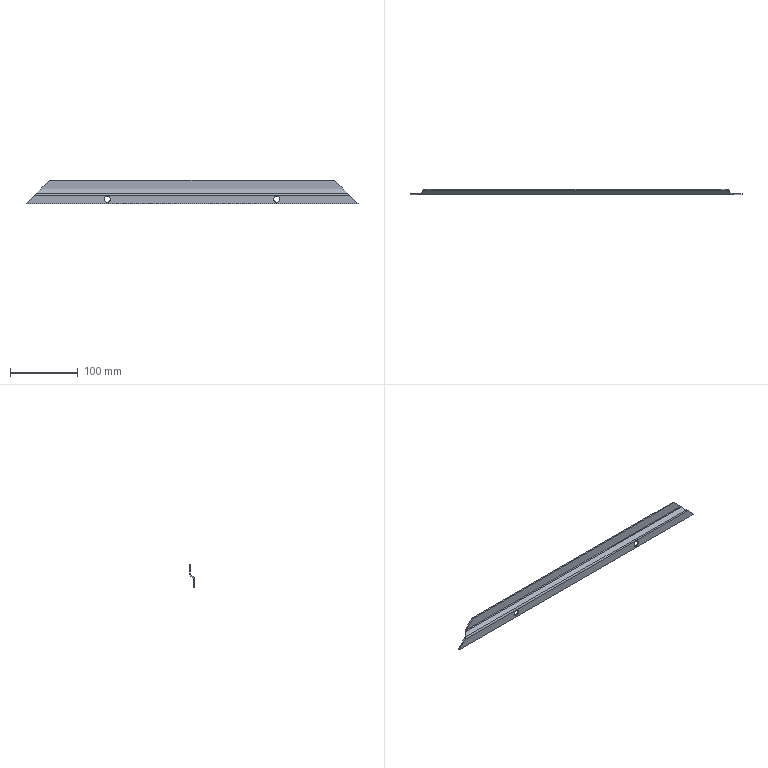Part | NX | features solid 2 | 1 solid | 26 faces | box 490 x 8.5 x 35 mm | volume 33694 mm3 | plane 14 | cylinder 8 | spline 4 | commonest cylinder face diameters 9 x4 4 x2 8 x2
STEP:
#1=CARTESIAN_POINT('',(-50.,-1613.,347.816));
#2=VERTEX_POINT('',#1);
#3=CARTESIAN_POINT('',(-50.,-1615.,347.816));
#4=VERTEX_POINT('',#3);
#5=CARTESIAN_POINT('',(-50.,-2104.322,347.816));
#6=DIRECTION('',(0.,1.,0.));
#7=VECTOR('',#6,1000.);
#8=LINE('',#5,#7);
#9=EDGE_CURVE('',#2,#4,#8,.F.);
#10=ORIENTED_EDGE('',*,*,#9,.T.);
#11=CARTESIAN_POINT('',(-50.,-1615.,338.816));
#12=VERTEX_POINT('',#11);
#13=CARTESIAN_POINT('',(-50.,-1615.,343.316));
#14=DIRECTION('',(0.,-1.,0.));
#15=DIRECTION('',(0.,0.,1.));
#16=AXIS2_PLACEMENT_3D('',#13,#14,#15);
#17=CIRCLE('',#16,4.5);
#18=EDGE_CURVE('',#4,#12,#17,.T.);
#19=ORIENTED_EDGE('',*,*,#18,.T.);
#20=CARTESIAN_POINT('',(-50.,-1613.,338.816));
#21=VERTEX_POINT('',#20);
#22=CARTESIAN_POINT('',(-50.,-2104.322,338.816));
#23=DIRECTION('',(0.,1.,0.));
#24=VECTOR('',#23,1000.);
#25=LINE('',#22,#24);
#26=EDGE_CURVE('',#12,#21,#25,.T.);
#27=ORIENTED_EDGE('',*,*,#26,.T.);
#28=CARTESIAN_POINT('',(-50.,-1613.,343.316));
#29=DIRECTION('',(0.,1.,0.));
#30=DIRECTION('',(-1.,0.,0.));
#31=AXIS2_PLACEMENT_3D('',#28,#29,#30);
#32=CIRCLE('',#31,4.5);
#33=EDGE_CURVE('',#21,#2,#32,.T.);
#34=ORIENTED_EDGE('',*,*,#33,.T.);
#35=EDGE_LOOP('',(#10,#19,#27,#34));
#36=FACE_BOUND('',#35,.T.);
#37=CARTESIAN_POINT('',(-50.,-2104.322,343.316));
#38=DIRECTION('',(0.,1.,0.));
#39=DIRECTION('',(0.,0.,-1.));
#40=AXIS2_PLACEMENT_3D('',#37,#38,#39);
#41=CYLINDRICAL_SURFACE('',#40,4.5);
#42=ADVANCED_FACE('',(#36),#41,.F.);
#43=CARTESIAN_POINT('',(200.,-1615.,347.816));
#44=VERTEX_POINT('',#43);
#45=CARTESIAN_POINT('',(200.,-1613.,347.816));
#46=VERTEX_POINT('',#45);
#47=CARTESIAN_POINT('',(200.,-2104.322,347.816));
#48=DIRECTION('',(0.,1.,0.));
#49=VECTOR('',#48,1000.);
#50=LINE('',#47,#49);
#51=EDGE_CURVE('',#44,#46,#50,.T.);
#52=ORIENTED_EDGE('',*,*,#51,.F.);
#53=CARTESIAN_POINT('',(200.,-1615.,338.816));
#54=VERTEX_POINT('',#53);
#55=CARTESIAN_POINT('',(200.,-1615.,343.316));
#56=DIRECTION('',(0.,-1.,0.));
#57=DIRECTION('',(0.,0.,1.));
#58=AXIS2_PLACEMENT_3D('',#55,#56,#57);
#59=CIRCLE('',#58,4.5);
#60=EDGE_CURVE('',#44,#54,#59,.T.);
#61=ORIENTED_EDGE('',*,*,#60,.T.);
#62=CARTESIAN_POINT('',(200.,-1613.,338.816));
#63=VERTEX_POINT('',#62);
#64=CARTESIAN_POINT('',(200.,-2104.322,338.816));
#65=DIRECTION('',(0.,1.,0.));
#66=VECTOR('',#65,1000.);
#67=LINE('',#64,#66);
#68=EDGE_CURVE('',#63,#54,#67,.F.);
#69=ORIENTED_EDGE('',*,*,#68,.F.);
#70=CARTESIAN_POINT('',(200.,-1613.,343.316));
#71=DIRECTION('',(0.,1.,0.));
#72=DIRECTION('',(-1.,0.,0.));
#73=AXIS2_PLACEMENT_3D('',#70,#71,#72);
#74=CIRCLE('',#73,4.5);
#75=EDGE_CURVE('',#63,#46,#74,.T.);
#76=ORIENTED_EDGE('',*,*,#75,.T.);
#77=EDGE_LOOP('',(#52,#61,#69,#76));
#78=FACE_BOUND('',#77,.T.);
#79=CARTESIAN_POINT('',(200.,-2104.322,343.316));
#80=DIRECTION('',(0.,1.,0.));
#81=DIRECTION('',(0.,0.,-1.));
#82=AXIS2_PLACEMENT_3D('',#79,#80,#81);
#83=CYLINDRICAL_SURFACE('',#82,4.5);
#84=ADVANCED_FACE('',(#78),#83,.F.);
#85=CARTESIAN_POINT('',(307.571,-1613.,348.745));
#86=VERTEX_POINT('',#85);
#87=CARTESIAN_POINT('',(307.571,-1615.,348.745));
#88=VERTEX_POINT('',#87);
#89=CARTESIAN_POINT('',(307.571,-1615.,348.745));
#90=DIRECTION('',(0.,-1.,0.));
#91=VECTOR('',#90,1000.);
#92=LINE('',#89,#91);
#93=EDGE_CURVE('',#86,#88,#92,.T.);
#94=ORIENTED_EDGE('',*,*,#93,.T.);
#95=CARTESIAN_POINT('',(320.,-1615.,336.316));
#96=VERTEX_POINT('',#95);
#97=CARTESIAN_POINT('',(-667.,-1615.,1323.316));
#98=DIRECTION('',(0.7071,0.,-0.7071));
#99=VECTOR('',#98,1000.);
#100=LINE('',#97,#99);
#101=EDGE_CURVE('',#88,#96,#100,.T.);
#102=ORIENTED_EDGE('',*,*,#101,.T.);
#103=CARTESIAN_POINT('',(320.,-1613.,336.316));
#104=VERTEX_POINT('',#103);
#105=CARTESIAN_POINT('',(320.,-1615.,336.316));
#106=DIRECTION('',(0.,-1.,0.));
#107=VECTOR('',#106,1000.);
#108=LINE('',#105,#107);
#109=EDGE_CURVE('',#104,#96,#108,.T.);
#110=ORIENTED_EDGE('',*,*,#109,.F.);
#111=CARTESIAN_POINT('',(-667.,-1613.,1323.316));
#112=DIRECTION('',(0.7071,0.,-0.7071));
#113=VECTOR('',#112,1000.);
#114=LINE('',#111,#113);
#115=EDGE_CURVE('',#86,#104,#114,.T.);
#116=ORIENTED_EDGE('',*,*,#115,.F.);
#117=EDGE_LOOP('',(#94,#102,#110,#116));
#118=FACE_BOUND('',#117,.T.);
#119=CARTESIAN_POINT('',(-667.,-1615.,1323.316));
#120=DIRECTION('',(-0.7071,0.,-0.7071));
#121=DIRECTION('',(-0.7071,0.,0.7071));
#122=AXIS2_PLACEMENT_3D('',#119,#120,#121);
#123=PLANE('',#122);
#124=ADVANCED_FACE('',(#118),#123,.F.);
#125=CARTESIAN_POINT('',(304.849,-1612.466,350.106));
#126=VERTEX_POINT('',#125);
#127=CARTESIAN_POINT('',(304.849,-1613.931,351.467));
#128=VERTEX_POINT('',#127);
#129=CARTESIAN_POINT('',(304.849,-1613.931,351.467));
#130=DIRECTION('',(0.,-0.7328,0.6805));
#131=VECTOR('',#130,1000.);
#132=LINE('',#129,#131);
#133=EDGE_CURVE('',#126,#128,#132,.T.);
#134=ORIENTED_EDGE('',*,*,#133,.T.);
#135=CARTESIAN_POINT('',(304.849,-1613.931,351.467));
#136=CARTESIAN_POINT('',(305.598,-1614.626,350.718));
#137=CARTESIAN_POINT('',(306.549,-1615.,349.767));
#138=CARTESIAN_POINT('',(307.571,-1615.,348.745));
#139=(BOUNDED_CURVE()B_SPLINE_CURVE(3,(#135,#136,#137,#138),.UNSPECIFIED.,.F.,.F.)B_SPLINE_CURVE_WITH_KNOTS((4,4),(3.964,4.712),.PIECEWISE_BEZIER_KNOTS.)CURVE()GEOMETRIC_REPRESENTATION_ITEM()RATIONAL_B_SPLINE_CURVE((1.,0.9539,0.9539,1.))REPRESENTATION_ITEM(''));
#140=EDGE_CURVE('',#128,#88,#139,.T.);
#141=ORIENTED_EDGE('',*,*,#140,.T.);
#142=ORIENTED_EDGE('',*,*,#93,.F.);
#143=CARTESIAN_POINT('',(304.849,-1612.466,350.106));
#144=CARTESIAN_POINT('',(305.598,-1612.813,349.732));
#145=CARTESIAN_POINT('',(306.549,-1613.,349.256));
#146=CARTESIAN_POINT('',(307.571,-1613.,348.745));
#147=(BOUNDED_CURVE()B_SPLINE_CURVE(3,(#143,#144,#145,#146),.UNSPECIFIED.,.F.,.F.)B_SPLINE_CURVE_WITH_KNOTS((4,4),(3.964,4.712),.PIECEWISE_BEZIER_KNOTS.)CURVE()GEOMETRIC_REPRESENTATION_ITEM()RATIONAL_B_SPLINE_CURVE((1.,0.9539,0.9539,1.))REPRESENTATION_ITEM(''));
#148=EDGE_CURVE('',#126,#86,#147,.T.);
#149=ORIENTED_EDGE('',*,*,#148,.F.);
#150=EDGE_LOOP('',(#134,#141,#142,#149));
#151=FACE_BOUND('',#150,.T.);
#152=CARTESIAN_POINT('',(304.849,-1613.931,351.467));
#153=CARTESIAN_POINT('',(304.849,-1613.443,351.014));
#154=CARTESIAN_POINT('',(304.849,-1612.954,350.56));
#155=CARTESIAN_POINT('',(304.849,-1612.466,350.106));
#156=CARTESIAN_POINT('',(305.579,-1614.609,350.737));
#157=CARTESIAN_POINT('',(305.579,-1614.007,350.405));
#158=CARTESIAN_POINT('',(305.579,-1613.406,350.073));
#159=CARTESIAN_POINT('',(305.579,-1612.804,349.741));
#160=CARTESIAN_POINT('',(306.524,-1615.,349.793));
#161=CARTESIAN_POINT('',(306.524,-1614.333,349.618));
#162=CARTESIAN_POINT('',(306.524,-1613.667,349.444));
#163=CARTESIAN_POINT('',(306.524,-1613.,349.269));
#164=CARTESIAN_POINT('',(307.571,-1615.,348.745));
#165=CARTESIAN_POINT('',(307.571,-1614.333,348.745));
#166=CARTESIAN_POINT('',(307.571,-1613.667,348.745));
#167=CARTESIAN_POINT('',(307.571,-1613.,348.745));
#168=(BOUNDED_SURFACE()B_SPLINE_SURFACE(3,3,((#152,#153,#154,#155),(#156,#157,#158,#159),(#160,#161,#162,#163),(#164,#165,#166,#167)),.UNSPECIFIED.,.F.,.F.,.F.)B_SPLINE_SURFACE_WITH_KNOTS((4,4),(4,4),(0.6518,0.75),(0.,1.),.PIECEWISE_BEZIER_KNOTS.)GEOMETRIC_REPRESENTATION_ITEM()RATIONAL_B_SPLINE_SURFACE(((0.5771,0.5771,0.5771,0.5771),(0.5257,0.5257,0.5257,0.5257),(0.5,0.5,0.5,0.5),(0.5,0.5,0.5,0.5)))REPRESENTATION_ITEM('')SURFACE());
#169=ADVANCED_FACE('',(#151),#168,.T.);
#170=CARTESIAN_POINT('',(299.576,-1607.569,355.38));
#171=VERTEX_POINT('',#170);
#172=CARTESIAN_POINT('',(299.576,-1609.034,356.741));
#173=VERTEX_POINT('',#172);
#174=CARTESIAN_POINT('',(299.576,-1609.034,356.741));
#175=DIRECTION('',(0.,-0.7328,0.6805));
#176=VECTOR('',#175,1000.);
#177=LINE('',#174,#176);
#178=EDGE_CURVE('',#171,#173,#177,.T.);
#179=ORIENTED_EDGE('',*,*,#178,.T.);
#180=CARTESIAN_POINT('',(-378.44,-979.448,1034.757));
#181=DIRECTION('',(0.5911,-0.5489,-0.5911));
#182=VECTOR('',#181,1000.);
#183=LINE('',#180,#182);
#184=EDGE_CURVE('',#173,#128,#183,.T.);
#185=ORIENTED_EDGE('',*,*,#184,.T.);
#186=ORIENTED_EDGE('',*,*,#133,.F.);
#187=CARTESIAN_POINT('',(-378.44,-977.983,1033.396));
#188=DIRECTION('',(0.5911,-0.5489,-0.5911));
#189=VECTOR('',#188,1000.);
#190=LINE('',#187,#189);
#191=EDGE_CURVE('',#171,#126,#190,.T.);
#192=ORIENTED_EDGE('',*,*,#191,.F.);
#193=EDGE_LOOP('',(#179,#185,#186,#192));
#194=FACE_BOUND('',#193,.T.);
#195=CARTESIAN_POINT('',(-378.44,-979.448,1034.757));
#196=DIRECTION('',(-0.8066,-0.4022,-0.4331));
#197=DIRECTION('',(-0.4731,0.,0.881));
#198=AXIS2_PLACEMENT_3D('',#195,#196,#197);
#199=PLANE('',#198);
#200=ADVANCED_FACE('',(#194),#199,.F.);
#201=CARTESIAN_POINT('',(298.215,-1606.5,358.102));
#202=VERTEX_POINT('',#201);
#203=CARTESIAN_POINT('',(298.215,-1608.5,358.102));
#204=VERTEX_POINT('',#203);
#205=CARTESIAN_POINT('',(298.215,-1608.5,358.102));
#206=DIRECTION('',(0.,-1.,0.));
#207=VECTOR('',#206,1000.);
#208=LINE('',#205,#207);
#209=EDGE_CURVE('',#202,#204,#208,.T.);
#210=ORIENTED_EDGE('',*,*,#209,.T.);
#211=CARTESIAN_POINT('',(298.215,-1608.5,358.102));
#212=CARTESIAN_POINT('',(298.726,-1608.5,357.591));
#213=CARTESIAN_POINT('',(299.201,-1608.687,357.115));
#214=CARTESIAN_POINT('',(299.576,-1609.034,356.741));
#215=(BOUNDED_CURVE()B_SPLINE_CURVE(3,(#211,#212,#213,#214),.UNSPECIFIED.,.F.,.F.)B_SPLINE_CURVE_WITH_KNOTS((4,4),(4.712,5.461),.PIECEWISE_BEZIER_KNOTS.)CURVE()GEOMETRIC_REPRESENTATION_ITEM()RATIONAL_B_SPLINE_CURVE((1.,0.9539,0.9539,1.))REPRESENTATION_ITEM(''));
#216=EDGE_CURVE('',#204,#173,#215,.T.);
#217=ORIENTED_EDGE('',*,*,#216,.T.);
#218=ORIENTED_EDGE('',*,*,#178,.F.);
#219=CARTESIAN_POINT('',(298.215,-1606.5,358.102));
#220=CARTESIAN_POINT('',(298.726,-1606.5,357.08));
#221=CARTESIAN_POINT('',(299.201,-1606.874,356.129));
#222=CARTESIAN_POINT('',(299.576,-1607.569,355.38));
#223=(BOUNDED_CURVE()B_SPLINE_CURVE(3,(#219,#220,#221,#222),.UNSPECIFIED.,.F.,.F.)B_SPLINE_CURVE_WITH_KNOTS((4,4),(4.712,5.461),.PIECEWISE_BEZIER_KNOTS.)CURVE()GEOMETRIC_REPRESENTATION_ITEM()RATIONAL_B_SPLINE_CURVE((1.,0.9539,0.9539,1.))REPRESENTATION_ITEM(''));
#224=EDGE_CURVE('',#202,#171,#223,.T.);
#225=ORIENTED_EDGE('',*,*,#224,.F.);
#226=EDGE_LOOP('',(#210,#217,#218,#225));
#227=FACE_BOUND('',#226,.T.);
#228=CARTESIAN_POINT('',(298.215,-1608.5,358.102));
#229=CARTESIAN_POINT('',(298.215,-1607.833,358.102));
#230=CARTESIAN_POINT('',(298.215,-1607.167,358.102));
#231=CARTESIAN_POINT('',(298.215,-1606.5,358.102));
#232=CARTESIAN_POINT('',(298.738,-1608.5,357.578));
#233=CARTESIAN_POINT('',(298.738,-1607.833,357.403));
#234=CARTESIAN_POINT('',(298.738,-1607.167,357.229));
#235=CARTESIAN_POINT('',(298.738,-1606.5,357.054));
#236=CARTESIAN_POINT('',(299.211,-1608.696,357.106));
#237=CARTESIAN_POINT('',(299.211,-1608.094,356.774));
#238=CARTESIAN_POINT('',(299.211,-1607.493,356.442));
#239=CARTESIAN_POINT('',(299.211,-1606.891,356.11));
#240=CARTESIAN_POINT('',(299.576,-1609.034,356.741));
#241=CARTESIAN_POINT('',(299.576,-1608.546,356.287));
#242=CARTESIAN_POINT('',(299.576,-1608.057,355.833));
#243=CARTESIAN_POINT('',(299.576,-1607.569,355.38));
#244=(BOUNDED_SURFACE()B_SPLINE_SURFACE(3,3,((#228,#229,#230,#231),(#232,#233,#234,#235),(#236,#237,#238,#239),(#240,#241,#242,#243)),.UNSPECIFIED.,.F.,.F.,.F.)B_SPLINE_SURFACE_WITH_KNOTS((4,4),(4,4),(0.75,0.8482),(0.,1.),.PIECEWISE_BEZIER_KNOTS.)GEOMETRIC_REPRESENTATION_ITEM()RATIONAL_B_SPLINE_SURFACE(((0.5,0.5,0.5,0.5),(0.5,0.5,0.5,0.5),(0.5257,0.5257,0.5257,0.5257),(0.5771,0.5771,0.5771,0.5771)))REPRESENTATION_ITEM('')SURFACE());
#245=ADVANCED_FACE('',(#227),#244,.T.);
#246=CARTESIAN_POINT('',(285.,-1606.5,371.316));
#247=VERTEX_POINT('',#246);
#248=CARTESIAN_POINT('',(285.,-1608.5,371.316));
#249=VERTEX_POINT('',#248);
#250=CARTESIAN_POINT('',(285.,-1608.5,371.316));
#251=DIRECTION('',(0.,-1.,0.));
#252=VECTOR('',#251,1000.);
#253=LINE('',#250,#252);
#254=EDGE_CURVE('',#247,#249,#253,.T.);
#255=ORIENTED_EDGE('',*,*,#254,.T.);
#256=CARTESIAN_POINT('',(-677.5,-1608.5,1333.816));
#257=DIRECTION('',(0.7071,0.,-0.7071));
#258=VECTOR('',#257,1000.);
#259=LINE('',#256,#258);
#260=EDGE_CURVE('',#249,#204,#259,.T.);
#261=ORIENTED_EDGE('',*,*,#260,.T.);
#262=ORIENTED_EDGE('',*,*,#209,.F.);
#263=CARTESIAN_POINT('',(-677.5,-1606.5,1333.816));
#264=DIRECTION('',(0.7071,0.,-0.7071));
#265=VECTOR('',#264,1000.);
#266=LINE('',#263,#265);
#267=EDGE_CURVE('',#247,#202,#266,.T.);
#268=ORIENTED_EDGE('',*,*,#267,.F.);
#269=EDGE_LOOP('',(#255,#261,#262,#268));
#270=FACE_BOUND('',#269,.T.);
#271=CARTESIAN_POINT('',(-677.5,-1608.5,1333.816));
#272=DIRECTION('',(-0.7071,0.,-0.7071));
#273=DIRECTION('',(-0.7071,0.,0.7071));
#274=AXIS2_PLACEMENT_3D('',#271,#272,#273);
#275=PLANE('',#274);
#276=ADVANCED_FACE('',(#270),#275,.F.);
#277=CARTESIAN_POINT('',(-170.,-1613.,336.316));
#278=VERTEX_POINT('',#277);
#279=CARTESIAN_POINT('',(-157.571,-1613.,348.745));
#280=VERTEX_POINT('',#279);
#281=CARTESIAN_POINT('',(-898.,-1613.,-391.684));
#282=DIRECTION('',(0.7071,0.,0.7071));
#283=VECTOR('',#282,1000.);
#284=LINE('',#281,#283);
#285=EDGE_CURVE('',#278,#280,#284,.T.);
#286=ORIENTED_EDGE('',*,*,#285,.F.);
#287=CARTESIAN_POINT('',(-170.,-1615.,336.316));
#288=VERTEX_POINT('',#287);
#289=CARTESIAN_POINT('',(-170.,-1615.,336.316));
#290=DIRECTION('',(0.,-1.,0.));
#291=VECTOR('',#290,1000.);
#292=LINE('',#289,#291);
#293=EDGE_CURVE('',#278,#288,#292,.T.);
#294=ORIENTED_EDGE('',*,*,#293,.T.);
#295=CARTESIAN_POINT('',(-157.571,-1615.,348.745));
#296=VERTEX_POINT('',#295);
#297=CARTESIAN_POINT('',(-898.,-1615.,-391.684));
#298=DIRECTION('',(0.7071,0.,0.7071));
#299=VECTOR('',#298,1000.);
#300=LINE('',#297,#299);
#301=EDGE_CURVE('',#288,#296,#300,.T.);
#302=ORIENTED_EDGE('',*,*,#301,.T.);
#303=CARTESIAN_POINT('',(-157.571,-1615.,348.745));
#304=DIRECTION('',(0.,-1.,0.));
#305=VECTOR('',#304,1000.);
#306=LINE('',#303,#305);
#307=EDGE_CURVE('',#280,#296,#306,.T.);
#308=ORIENTED_EDGE('',*,*,#307,.F.);
#309=EDGE_LOOP('',(#286,#294,#302,#308));
#310=FACE_BOUND('',#309,.T.);
#311=CARTESIAN_POINT('',(-898.,-1615.,-391.684));
#312=DIRECTION('',(0.7071,0.,-0.7071));
#313=DIRECTION('',(0.,-1.,0.));
#314=AXIS2_PLACEMENT_3D('',#311,#312,#313);
#315=PLANE('',#314);
#316=ADVANCED_FACE('',(#310),#315,.F.);
#317=CARTESIAN_POINT('',(-148.215,-1606.5,358.102));
#318=VERTEX_POINT('',#317);
#319=CARTESIAN_POINT('',(-148.215,-1608.5,358.102));
#320=VERTEX_POINT('',#319);
#321=CARTESIAN_POINT('',(-148.215,-1608.5,358.102));
#322=DIRECTION('',(0.,-1.,0.));
#323=VECTOR('',#322,1000.);
#324=LINE('',#321,#323);
#325=EDGE_CURVE('',#318,#320,#324,.T.);
#326=ORIENTED_EDGE('',*,*,#325,.T.);
#327=CARTESIAN_POINT('',(-135.,-1608.5,371.316));
#328=VERTEX_POINT('',#327);
#329=CARTESIAN_POINT('',(-887.5,-1608.5,-381.184));
#330=DIRECTION('',(0.7071,0.,0.7071));
#331=VECTOR('',#330,1000.);
#332=LINE('',#329,#331);
#333=EDGE_CURVE('',#320,#328,#332,.T.);
#334=ORIENTED_EDGE('',*,*,#333,.T.);
#335=CARTESIAN_POINT('',(-135.,-1606.5,371.316));
#336=VERTEX_POINT('',#335);
#337=CARTESIAN_POINT('',(-135.,-1608.5,371.316));
#338=DIRECTION('',(0.,-1.,0.));
#339=VECTOR('',#338,1000.);
#340=LINE('',#337,#339);
#341=EDGE_CURVE('',#336,#328,#340,.T.);
#342=ORIENTED_EDGE('',*,*,#341,.F.);
#343=CARTESIAN_POINT('',(-887.5,-1606.5,-381.184));
#344=DIRECTION('',(0.7071,0.,0.7071));
#345=VECTOR('',#344,1000.);
#346=LINE('',#343,#345);
#347=EDGE_CURVE('',#318,#336,#346,.T.);
#348=ORIENTED_EDGE('',*,*,#347,.F.);
#349=EDGE_LOOP('',(#326,#334,#342,#348));
#350=FACE_BOUND('',#349,.T.);
#351=CARTESIAN_POINT('',(-887.5,-1608.5,-381.184));
#352=DIRECTION('',(0.7071,0.,-0.7071));
#353=DIRECTION('',(0.,-1.,0.));
#354=AXIS2_PLACEMENT_3D('',#351,#352,#353);
#355=PLANE('',#354);
#356=ADVANCED_FACE('',(#350),#355,.F.);
#357=CARTESIAN_POINT('',(-149.576,-1607.569,355.38));
#358=VERTEX_POINT('',#357);
#359=CARTESIAN_POINT('',(-149.576,-1609.034,356.741));
#360=VERTEX_POINT('',#359);
#361=CARTESIAN_POINT('',(-149.576,-1609.034,356.741));
#362=DIRECTION('',(0.,-0.7328,0.6805));
#363=VECTOR('',#362,1000.);
#364=LINE('',#361,#363);
#365=EDGE_CURVE('',#358,#360,#364,.T.);
#366=ORIENTED_EDGE('',*,*,#365,.T.);
#367=CARTESIAN_POINT('',(-149.576,-1609.034,356.741));
#368=CARTESIAN_POINT('',(-149.201,-1608.687,357.115));
#369=CARTESIAN_POINT('',(-148.726,-1608.5,357.591));
#370=CARTESIAN_POINT('',(-148.215,-1608.5,358.102));
#371=(BOUNDED_CURVE()B_SPLINE_CURVE(3,(#367,#368,#369,#370),.UNSPECIFIED.,.F.,.F.)B_SPLINE_CURVE_WITH_KNOTS((4,4),(3.964,4.712),.PIECEWISE_BEZIER_KNOTS.)CURVE()GEOMETRIC_REPRESENTATION_ITEM()RATIONAL_B_SPLINE_CURVE((1.,0.9539,0.9539,1.))REPRESENTATION_ITEM(''));
#372=EDGE_CURVE('',#360,#320,#371,.T.);
#373=ORIENTED_EDGE('',*,*,#372,.T.);
#374=ORIENTED_EDGE('',*,*,#325,.F.);
#375=CARTESIAN_POINT('',(-149.576,-1607.569,355.38));
#376=CARTESIAN_POINT('',(-149.201,-1606.874,356.129));
#377=CARTESIAN_POINT('',(-148.726,-1606.5,357.08));
#378=CARTESIAN_POINT('',(-148.215,-1606.5,358.102));
#379=(BOUNDED_CURVE()B_SPLINE_CURVE(3,(#375,#376,#377,#378),.UNSPECIFIED.,.F.,.F.)B_SPLINE_CURVE_WITH_KNOTS((4,4),(3.964,4.712),.PIECEWISE_BEZIER_KNOTS.)CURVE()GEOMETRIC_REPRESENTATION_ITEM()RATIONAL_B_SPLINE_CURVE((1.,0.9539,0.9539,1.))REPRESENTATION_ITEM(''));
#380=EDGE_CURVE('',#358,#318,#379,.T.);
#381=ORIENTED_EDGE('',*,*,#380,.F.);
#382=EDGE_LOOP('',(#366,#373,#374,#381));
#383=FACE_BOUND('',#382,.T.);
#384=CARTESIAN_POINT('',(-149.576,-1609.034,356.741));
#385=CARTESIAN_POINT('',(-149.576,-1608.546,356.287));
#386=CARTESIAN_POINT('',(-149.576,-1608.057,355.833));
#387=CARTESIAN_POINT('',(-149.576,-1607.569,355.38));
#388=CARTESIAN_POINT('',(-149.211,-1608.696,357.106));
#389=CARTESIAN_POINT('',(-149.211,-1608.094,356.774));
#390=CARTESIAN_POINT('',(-149.211,-1607.493,356.442));
#391=CARTESIAN_POINT('',(-149.211,-1606.891,356.11));
#392=CARTESIAN_POINT('',(-148.738,-1608.5,357.578));
#393=CARTESIAN_POINT('',(-148.738,-1607.833,357.403));
#394=CARTESIAN_POINT('',(-148.738,-1607.167,357.229));
#395=CARTESIAN_POINT('',(-148.738,-1606.5,357.054));
#396=CARTESIAN_POINT('',(-148.215,-1608.5,358.102));
#397=CARTESIAN_POINT('',(-148.215,-1607.833,358.102));
#398=CARTESIAN_POINT('',(-148.215,-1607.167,358.102));
#399=CARTESIAN_POINT('',(-148.215,-1606.5,358.102));
#400=(BOUNDED_SURFACE()B_SPLINE_SURFACE(3,3,((#384,#385,#386,#387),(#388,#389,#390,#391),(#392,#393,#394,#395),(#396,#397,#398,#399)),.UNSPECIFIED.,.F.,.F.,.F.)B_SPLINE_SURFACE_WITH_KNOTS((4,4),(4,4),(0.6518,0.75),(0.,1.),.PIECEWISE_BEZIER_KNOTS.)GEOMETRIC_REPRESENTATION_ITEM()RATIONAL_B_SPLINE_SURFACE(((0.5771,0.5771,0.5771,0.5771),(0.5257,0.5257,0.5257,0.5257),(0.5,0.5,0.5,0.5),(0.5,0.5,0.5,0.5)))REPRESENTATION_ITEM('')SURFACE());
#401=ADVANCED_FACE('',(#383),#400,.T.);
#402=CARTESIAN_POINT('',(-154.849,-1612.466,350.106));
#403=VERTEX_POINT('',#402);
#404=CARTESIAN_POINT('',(-154.849,-1613.931,351.467));
#405=VERTEX_POINT('',#404);
#406=CARTESIAN_POINT('',(-154.849,-1613.931,351.467));
#407=DIRECTION('',(0.,-0.7328,0.6805));
#408=VECTOR('',#407,1000.);
#409=LINE('',#406,#408);
#410=EDGE_CURVE('',#403,#405,#409,.T.);
#411=ORIENTED_EDGE('',*,*,#410,.T.);
#412=CARTESIAN_POINT('',(-669.92,-2092.211,-163.604));
#413=DIRECTION('',(0.5911,0.5489,0.5911));
#414=VECTOR('',#413,1000.);
#415=LINE('',#412,#414);
#416=EDGE_CURVE('',#405,#360,#415,.T.);
#417=ORIENTED_EDGE('',*,*,#416,.T.);
#418=ORIENTED_EDGE('',*,*,#365,.F.);
#419=CARTESIAN_POINT('',(-669.92,-2090.746,-164.964));
#420=DIRECTION('',(0.5911,0.5489,0.5911));
#421=VECTOR('',#420,1000.);
#422=LINE('',#419,#421);
#423=EDGE_CURVE('',#403,#358,#422,.T.);
#424=ORIENTED_EDGE('',*,*,#423,.F.);
#425=EDGE_LOOP('',(#411,#417,#418,#424));
#426=FACE_BOUND('',#425,.T.);
#427=CARTESIAN_POINT('',(-669.92,-2092.211,-163.604));
#428=DIRECTION('',(0.8066,-0.4022,-0.4331));
#429=DIRECTION('',(0.,-0.7328,0.6805));
#430=AXIS2_PLACEMENT_3D('',#427,#428,#429);
#431=PLANE('',#430);
#432=ADVANCED_FACE('',(#426),#431,.F.);
#433=ORIENTED_EDGE('',*,*,#307,.T.);
#434=CARTESIAN_POINT('',(-157.571,-1615.,348.745));
#435=CARTESIAN_POINT('',(-156.549,-1615.,349.767));
#436=CARTESIAN_POINT('',(-155.598,-1614.626,350.718));
#437=CARTESIAN_POINT('',(-154.849,-1613.931,351.467));
#438=(BOUNDED_CURVE()B_SPLINE_CURVE(3,(#434,#435,#436,#437),.UNSPECIFIED.,.F.,.F.)B_SPLINE_CURVE_WITH_KNOTS((4,4),(4.712,5.461),.PIECEWISE_BEZIER_KNOTS.)CURVE()GEOMETRIC_REPRESENTATION_ITEM()RATIONAL_B_SPLINE_CURVE((1.,0.9539,0.9539,1.))REPRESENTATION_ITEM(''));
#439=EDGE_CURVE('',#296,#405,#438,.T.);
#440=ORIENTED_EDGE('',*,*,#439,.T.);
#441=ORIENTED_EDGE('',*,*,#410,.F.);
#442=CARTESIAN_POINT('',(-157.571,-1613.,348.745));
#443=CARTESIAN_POINT('',(-156.549,-1613.,349.256));
#444=CARTESIAN_POINT('',(-155.598,-1612.813,349.732));
#445=CARTESIAN_POINT('',(-154.849,-1612.466,350.106));
#446=(BOUNDED_CURVE()B_SPLINE_CURVE(3,(#442,#443,#444,#445),.UNSPECIFIED.,.F.,.F.)B_SPLINE_CURVE_WITH_KNOTS((4,4),(4.712,5.461),.PIECEWISE_BEZIER_KNOTS.)CURVE()GEOMETRIC_REPRESENTATION_ITEM()RATIONAL_B_SPLINE_CURVE((1.,0.9539,0.9539,1.))REPRESENTATION_ITEM(''));
#447=EDGE_CURVE('',#280,#403,#446,.T.);
#448=ORIENTED_EDGE('',*,*,#447,.F.);
#449=EDGE_LOOP('',(#433,#440,#441,#448));
#450=FACE_BOUND('',#449,.T.);
#451=CARTESIAN_POINT('',(-157.571,-1615.,348.745));
#452=CARTESIAN_POINT('',(-157.571,-1614.333,348.745));
#453=CARTESIAN_POINT('',(-157.571,-1613.667,348.745));
#454=CARTESIAN_POINT('',(-157.571,-1613.,348.745));
#455=CARTESIAN_POINT('',(-156.524,-1615.,349.793));
#456=CARTESIAN_POINT('',(-156.524,-1614.333,349.618));
#457=CARTESIAN_POINT('',(-156.524,-1613.667,349.444));
#458=CARTESIAN_POINT('',(-156.524,-1613.,349.269));
#459=CARTESIAN_POINT('',(-155.579,-1614.609,350.737));
#460=CARTESIAN_POINT('',(-155.579,-1614.007,350.405));
#461=CARTESIAN_POINT('',(-155.579,-1613.406,350.073));
#462=CARTESIAN_POINT('',(-155.579,-1612.804,349.741));
#463=CARTESIAN_POINT('',(-154.849,-1613.931,351.467));
#464=CARTESIAN_POINT('',(-154.849,-1613.443,351.014));
#465=CARTESIAN_POINT('',(-154.849,-1612.954,350.56));
#466=CARTESIAN_POINT('',(-154.849,-1612.466,350.106));
#467=(BOUNDED_SURFACE()B_SPLINE_SURFACE(3,3,((#451,#452,#453,#454),(#455,#456,#457,#458),(#459,#460,#461,#462),(#463,#464,#465,#466)),.UNSPECIFIED.,.F.,.F.,.F.)B_SPLINE_SURFACE_WITH_KNOTS((4,4),(4,4),(0.75,0.8482),(0.,1.),.PIECEWISE_BEZIER_KNOTS.)GEOMETRIC_REPRESENTATION_ITEM()RATIONAL_B_SPLINE_SURFACE(((0.5,0.5,0.5,0.5),(0.5,0.5,0.5,0.5),(0.5257,0.5257,0.5257,0.5257),(0.5771,0.5771,0.5771,0.5771)))REPRESENTATION_ITEM('')SURFACE());
#468=ADVANCED_FACE('',(#450),#467,.T.);
#469=ORIENTED_EDGE('',*,*,#75,.F.);
#470=CARTESIAN_POINT('',(200.,-1613.,343.316));
#471=DIRECTION('',(0.,1.,0.));
#472=DIRECTION('',(-1.,0.,0.));
#473=AXIS2_PLACEMENT_3D('',#470,#471,#472);
#474=CIRCLE('',#473,4.5);
#475=EDGE_CURVE('',#46,#63,#474,.T.);
#476=ORIENTED_EDGE('',*,*,#475,.F.);
#477=EDGE_LOOP('',(#469,#476));
#478=FACE_BOUND('',#477,.T.);
#479=ORIENTED_EDGE('',*,*,#33,.F.);
#480=CARTESIAN_POINT('',(-50.,-1613.,343.316));
#481=DIRECTION('',(0.,1.,0.));
#482=DIRECTION('',(-1.,0.,0.));
#483=AXIS2_PLACEMENT_3D('',#480,#481,#482);
#484=CIRCLE('',#483,4.5);
#485=EDGE_CURVE('',#2,#21,#484,.T.);
#486=ORIENTED_EDGE('',*,*,#485,.F.);
#487=EDGE_LOOP('',(#479,#486));
#488=FACE_BOUND('',#487,.T.);
#489=CARTESIAN_POINT('',(-1640.,-1613.,348.745));
#490=DIRECTION('',(1.,0.,0.));
#491=VECTOR('',#490,1000.);
#492=LINE('',#489,#491);
#493=EDGE_CURVE('',#280,#86,#492,.T.);
#494=ORIENTED_EDGE('',*,*,#493,.T.);
#495=ORIENTED_EDGE('',*,*,#115,.T.);
#496=CARTESIAN_POINT('',(-1640.,-1613.,336.316));
#497=DIRECTION('',(1.,0.,0.));
#498=VECTOR('',#497,1000.);
#499=LINE('',#496,#498);
#500=EDGE_CURVE('',#278,#104,#499,.T.);
#501=ORIENTED_EDGE('',*,*,#500,.F.);
#502=ORIENTED_EDGE('',*,*,#285,.T.);
#503=EDGE_LOOP('',(#494,#495,#501,#502));
#504=FACE_BOUND('',#503,.T.);
#505=CARTESIAN_POINT('',(-1640.,-1613.,350.316));
#506=DIRECTION('',(0.,-1.,0.));
#507=DIRECTION('',(0.,0.,-1.));
#508=AXIS2_PLACEMENT_3D('',#505,#506,#507);
#509=PLANE('',#508);
#510=ADVANCED_FACE('',(#478,#488,#504),#509,.F.);
#511=CARTESIAN_POINT('',(-1640.,-1612.466,350.106));
#512=DIRECTION('',(1.,0.,0.));
#513=VECTOR('',#512,1000.);
#514=LINE('',#511,#513);
#515=EDGE_CURVE('',#403,#126,#514,.T.);
#516=ORIENTED_EDGE('',*,*,#515,.T.);
#517=ORIENTED_EDGE('',*,*,#148,.T.);
#518=ORIENTED_EDGE('',*,*,#493,.F.);
#519=ORIENTED_EDGE('',*,*,#447,.T.);
#520=EDGE_LOOP('',(#516,#517,#518,#519));
#521=FACE_BOUND('',#520,.T.);
#522=CARTESIAN_POINT('',(-1640.,-1611.,348.745));
#523=DIRECTION('',(1.,0.,0.));
#524=DIRECTION('',(0.,-1.,0.));
#525=AXIS2_PLACEMENT_3D('',#522,#523,#524);
#526=CYLINDRICAL_SURFACE('',#525,2.);
#527=ADVANCED_FACE('',(#521),#526,.F.);
#528=CARTESIAN_POINT('',(-1640.,-1607.569,355.38));
#529=DIRECTION('',(1.,0.,0.));
#530=VECTOR('',#529,1000.);
#531=LINE('',#528,#530);
#532=EDGE_CURVE('',#358,#171,#531,.T.);
#533=ORIENTED_EDGE('',*,*,#532,.T.);
#534=ORIENTED_EDGE('',*,*,#191,.T.);
#535=ORIENTED_EDGE('',*,*,#515,.F.);
#536=ORIENTED_EDGE('',*,*,#423,.T.);
#537=EDGE_LOOP('',(#533,#534,#535,#536));
#538=FACE_BOUND('',#537,.T.);
#539=CARTESIAN_POINT('',(-1640.,-1607.034,355.955));
#540=DIRECTION('',(0.,-0.7328,0.6805));
#541=DIRECTION('',(-1.,0.,0.));
#542=AXIS2_PLACEMENT_3D('',#539,#540,#541);
#543=PLANE('',#542);
#544=ADVANCED_FACE('',(#538),#543,.F.);
#545=CARTESIAN_POINT('',(-1640.,-1606.5,358.102));
#546=DIRECTION('',(1.,0.,0.));
#547=VECTOR('',#546,1000.);
#548=LINE('',#545,#547);
#549=EDGE_CURVE('',#318,#202,#548,.T.);
#550=ORIENTED_EDGE('',*,*,#549,.T.);
#551=ORIENTED_EDGE('',*,*,#224,.T.);
#552=ORIENTED_EDGE('',*,*,#532,.F.);
#553=ORIENTED_EDGE('',*,*,#380,.T.);
#554=EDGE_LOOP('',(#550,#551,#552,#553));
#555=FACE_BOUND('',#554,.T.);
#556=CARTESIAN_POINT('',(-1640.,-1610.5,358.102));
#557=DIRECTION('',(1.,0.,0.));
#558=DIRECTION('',(0.,-1.,0.));
#559=AXIS2_PLACEMENT_3D('',#556,#557,#558);
#560=CYLINDRICAL_SURFACE('',#559,4.);
#561=ADVANCED_FACE('',(#555),#560,.T.);
#562=CARTESIAN_POINT('',(-1640.,-1606.5,371.316));
#563=DIRECTION('',(1.,0.,0.));
#564=VECTOR('',#563,1000.);
#565=LINE('',#562,#564);
#566=EDGE_CURVE('',#336,#247,#565,.T.);
#567=ORIENTED_EDGE('',*,*,#566,.T.);
#568=ORIENTED_EDGE('',*,*,#267,.T.);
#569=ORIENTED_EDGE('',*,*,#549,.F.);
#570=ORIENTED_EDGE('',*,*,#347,.T.);
#571=EDGE_LOOP('',(#567,#568,#569,#570));
#572=FACE_BOUND('',#571,.T.);
#573=CARTESIAN_POINT('',(-1640.,-1606.5,371.316));
#574=DIRECTION('',(0.,-1.,0.));
#575=DIRECTION('',(0.,0.,-1.));
#576=AXIS2_PLACEMENT_3D('',#573,#574,#575);
#577=PLANE('',#576);
#578=ADVANCED_FACE('',(#572),#577,.F.);
#579=ORIENTED_EDGE('',*,*,#254,.F.);
#580=ORIENTED_EDGE('',*,*,#566,.F.);
#581=ORIENTED_EDGE('',*,*,#341,.T.);
#582=CARTESIAN_POINT('',(-1640.,-1608.5,371.316));
#583=DIRECTION('',(1.,0.,0.));
#584=VECTOR('',#583,1000.);
#585=LINE('',#582,#584);
#586=EDGE_CURVE('',#328,#249,#585,.T.);
#587=ORIENTED_EDGE('',*,*,#586,.T.);
#588=EDGE_LOOP('',(#579,#580,#581,#587));
#589=FACE_BOUND('',#588,.T.);
#590=CARTESIAN_POINT('',(-1640.,-1608.5,371.316));
#591=DIRECTION('',(0.,0.,-1.));
#592=DIRECTION('',(0.,-1.,0.));
#593=AXIS2_PLACEMENT_3D('',#590,#591,#592);
#594=PLANE('',#593);
#595=ADVANCED_FACE('',(#589),#594,.F.);
#596=CARTESIAN_POINT('',(200.,-1615.,343.316));
#597=DIRECTION('',(0.,-1.,0.));
#598=DIRECTION('',(0.,0.,1.));
#599=AXIS2_PLACEMENT_3D('',#596,#597,#598);
#600=CIRCLE('',#599,4.5);
#601=EDGE_CURVE('',#54,#44,#600,.T.);
#602=ORIENTED_EDGE('',*,*,#601,.F.);
#603=ORIENTED_EDGE('',*,*,#60,.F.);
#604=EDGE_LOOP('',(#602,#603));
#605=FACE_BOUND('',#604,.T.);
#606=CARTESIAN_POINT('',(-50.,-1615.,343.316));
#607=DIRECTION('',(0.,-1.,0.));
#608=DIRECTION('',(0.,0.,1.));
#609=AXIS2_PLACEMENT_3D('',#606,#607,#608);
#610=CIRCLE('',#609,4.5);
#611=EDGE_CURVE('',#12,#4,#610,.T.);
#612=ORIENTED_EDGE('',*,*,#611,.F.);
#613=ORIENTED_EDGE('',*,*,#18,.F.);
#614=EDGE_LOOP('',(#612,#613));
#615=FACE_BOUND('',#614,.T.);
#616=ORIENTED_EDGE('',*,*,#101,.F.);
#617=CARTESIAN_POINT('',(-1640.,-1615.,348.745));
#618=DIRECTION('',(1.,0.,0.));
#619=VECTOR('',#618,1000.);
#620=LINE('',#617,#619);
#621=EDGE_CURVE('',#296,#88,#620,.T.);
#622=ORIENTED_EDGE('',*,*,#621,.F.);
#623=ORIENTED_EDGE('',*,*,#301,.F.);
#624=CARTESIAN_POINT('',(-1640.,-1615.,336.316));
#625=DIRECTION('',(1.,0.,0.));
#626=VECTOR('',#625,1000.);
#627=LINE('',#624,#626);
#628=EDGE_CURVE('',#288,#96,#627,.T.);
#629=ORIENTED_EDGE('',*,*,#628,.T.);
#630=EDGE_LOOP('',(#616,#622,#623,#629));
#631=FACE_BOUND('',#630,.T.);
#632=CARTESIAN_POINT('',(-1640.,-1615.,350.316));
#633=DIRECTION('',(0.,-1.,0.));
#634=DIRECTION('',(0.,0.,-1.));
#635=AXIS2_PLACEMENT_3D('',#632,#633,#634);
#636=PLANE('',#635);
#637=ADVANCED_FACE('',(#605,#615,#631),#636,.T.);
#638=ORIENTED_EDGE('',*,*,#140,.F.);
#639=CARTESIAN_POINT('',(-1640.,-1613.931,351.467));
#640=DIRECTION('',(1.,0.,0.));
#641=VECTOR('',#640,1000.);
#642=LINE('',#639,#641);
#643=EDGE_CURVE('',#405,#128,#642,.T.);
#644=ORIENTED_EDGE('',*,*,#643,.F.);
#645=ORIENTED_EDGE('',*,*,#439,.F.);
#646=ORIENTED_EDGE('',*,*,#621,.T.);
#647=EDGE_LOOP('',(#638,#644,#645,#646));
#648=FACE_BOUND('',#647,.T.);
#649=CARTESIAN_POINT('',(-1640.,-1611.,348.745));
#650=DIRECTION('',(1.,0.,0.));
#651=DIRECTION('',(0.,-1.,0.));
#652=AXIS2_PLACEMENT_3D('',#649,#650,#651);
#653=CYLINDRICAL_SURFACE('',#652,4.);
#654=ADVANCED_FACE('',(#648),#653,.T.);
#655=ORIENTED_EDGE('',*,*,#184,.F.);
#656=CARTESIAN_POINT('',(-1640.,-1609.034,356.741));
#657=DIRECTION('',(1.,0.,0.));
#658=VECTOR('',#657,1000.);
#659=LINE('',#656,#658);
#660=EDGE_CURVE('',#360,#173,#659,.T.);
#661=ORIENTED_EDGE('',*,*,#660,.F.);
#662=ORIENTED_EDGE('',*,*,#416,.F.);
#663=ORIENTED_EDGE('',*,*,#643,.T.);
#664=EDGE_LOOP('',(#655,#661,#662,#663));
#665=FACE_BOUND('',#664,.T.);
#666=CARTESIAN_POINT('',(-1640.,-1608.5,357.316));
#667=DIRECTION('',(0.,-0.7328,0.6805));
#668=DIRECTION('',(-1.,0.,0.));
#669=AXIS2_PLACEMENT_3D('',#666,#667,#668);
#670=PLANE('',#669);
#671=ADVANCED_FACE('',(#665),#670,.T.);
#672=ORIENTED_EDGE('',*,*,#216,.F.);
#673=CARTESIAN_POINT('',(-1640.,-1608.5,358.102));
#674=DIRECTION('',(1.,0.,0.));
#675=VECTOR('',#674,1000.);
#676=LINE('',#673,#675);
#677=EDGE_CURVE('',#320,#204,#676,.T.);
#678=ORIENTED_EDGE('',*,*,#677,.F.);
#679=ORIENTED_EDGE('',*,*,#372,.F.);
#680=ORIENTED_EDGE('',*,*,#660,.T.);
#681=EDGE_LOOP('',(#672,#678,#679,#680));
#682=FACE_BOUND('',#681,.T.);
#683=CARTESIAN_POINT('',(-1640.,-1610.5,358.102));
#684=DIRECTION('',(1.,0.,0.));
#685=DIRECTION('',(0.,-1.,0.));
#686=AXIS2_PLACEMENT_3D('',#683,#684,#685);
#687=CYLINDRICAL_SURFACE('',#686,2.);
#688=ADVANCED_FACE('',(#682),#687,.F.);
#689=ORIENTED_EDGE('',*,*,#260,.F.);
#690=ORIENTED_EDGE('',*,*,#586,.F.);
#691=ORIENTED_EDGE('',*,*,#333,.F.);
#692=ORIENTED_EDGE('',*,*,#677,.T.);
#693=EDGE_LOOP('',(#689,#690,#691,#692));
#694=FACE_BOUND('',#693,.T.);
#695=CARTESIAN_POINT('',(-1640.,-1608.5,371.316));
#696=DIRECTION('',(0.,-1.,0.));
#697=DIRECTION('',(0.,0.,-1.));
#698=AXIS2_PLACEMENT_3D('',#695,#696,#697);
#699=PLANE('',#698);
#700=ADVANCED_FACE('',(#694),#699,.T.);
#701=ORIENTED_EDGE('',*,*,#109,.T.);
#702=ORIENTED_EDGE('',*,*,#628,.F.);
#703=ORIENTED_EDGE('',*,*,#293,.F.);
#704=ORIENTED_EDGE('',*,*,#500,.T.);
#705=EDGE_LOOP('',(#701,#702,#703,#704));
#706=FACE_BOUND('',#705,.T.);
#707=CARTESIAN_POINT('',(-1640.,-1615.,336.316));
#708=DIRECTION('',(0.,0.,-1.));
#709=DIRECTION('',(0.,-1.,0.));
#710=AXIS2_PLACEMENT_3D('',#707,#708,#709);
#711=PLANE('',#710);
#712=ADVANCED_FACE('',(#706),#711,.T.);
#713=ORIENTED_EDGE('',*,*,#601,.T.);
#714=ORIENTED_EDGE('',*,*,#51,.T.);
#715=ORIENTED_EDGE('',*,*,#475,.T.);
#716=ORIENTED_EDGE('',*,*,#68,.T.);
#717=EDGE_LOOP('',(#713,#714,#715,#716));
#718=FACE_BOUND('',#717,.T.);
#719=CARTESIAN_POINT('',(200.,-2104.322,343.316));
#720=DIRECTION('',(0.,1.,0.));
#721=DIRECTION('',(0.,0.,-1.));
#722=AXIS2_PLACEMENT_3D('',#719,#720,#721);
#723=CYLINDRICAL_SURFACE('',#722,4.5);
#724=ADVANCED_FACE('',(#718),#723,.F.);
#725=ORIENTED_EDGE('',*,*,#611,.T.);
#726=ORIENTED_EDGE('',*,*,#9,.F.);
#727=ORIENTED_EDGE('',*,*,#485,.T.);
#728=ORIENTED_EDGE('',*,*,#26,.F.);
#729=EDGE_LOOP('',(#725,#726,#727,#728));
#730=FACE_BOUND('',#729,.T.);
#731=CARTESIAN_POINT('',(-50.,-2104.322,343.316));
#732=DIRECTION('',(0.,1.,0.));
#733=DIRECTION('',(0.,0.,-1.));
#734=AXIS2_PLACEMENT_3D('',#731,#732,#733);
#735=CYLINDRICAL_SURFACE('',#734,4.5);
#736=ADVANCED_FACE('',(#730),#735,.F.);
#737=CLOSED_SHELL('',(#42,#84,#124,#169,#200,#245,#276,#316,#356,#401,#432,#468,#510,#527,#544,#561,#578,#595,#637,#654,#671,#688,#700,#712,#724,#736));
#738=MANIFOLD_SOLID_BREP('',#737);
#739=(LENGTH_UNIT()NAMED_UNIT(*)SI_UNIT(.MILLI.,.METRE.));
#740=UNCERTAINTY_MEASURE_WITH_UNIT(LENGTH_MEASURE(0.00001),#739,'','');
#741=(NAMED_UNIT(*)PLANE_ANGLE_UNIT()SI_UNIT($,.RADIAN.));
#742=(NAMED_UNIT(*)SI_UNIT($,.STERADIAN.)SOLID_ANGLE_UNIT());
#743=(GEOMETRIC_REPRESENTATION_CONTEXT(3)GLOBAL_UNCERTAINTY_ASSIGNED_CONTEXT((#740))GLOBAL_UNIT_ASSIGNED_CONTEXT((#739,#741,#742))REPRESENTATION_CONTEXT('',''));
#744=ADVANCED_BREP_SHAPE_REPRESENTATION('',(#738),#743);